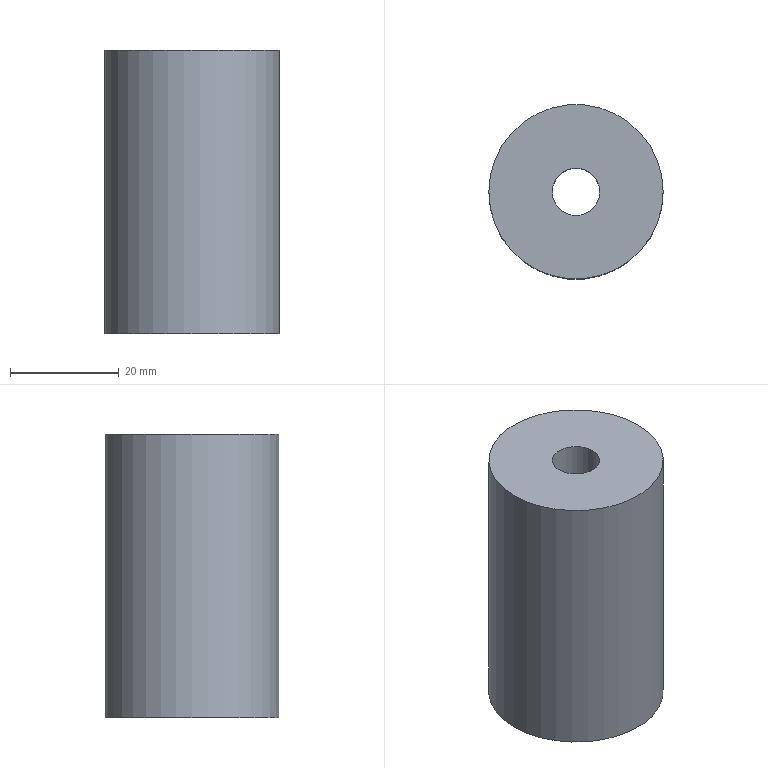Part | STEP file | 1_id1474_x_t | 1 solid | 6 faces | box 32 x 32 x 52.035 mm | volume 37231 mm3 | cylinder 3 | plane 3 | commonest cylinder face diameters 8.7 x1 15 x1 32 x1
STEP:
#1=CARTESIAN_POINT('',(0.,0.,0.));
#2=DIRECTION('',(0.,0.,1.));
#3=DIRECTION('',(1.,0.,0.));
#4=AXIS2_PLACEMENT_3D('',#1,#2,#3);
#5=CARTESIAN_POINT('',(238.925,-3.5,100.11));
#6=VERTEX_POINT('',#5);
#7=CARTESIAN_POINT('',(206.925,-3.5,100.11));
#8=VERTEX_POINT('',#7);
#9=CARTESIAN_POINT('',(222.925,-3.5,100.11));
#10=DIRECTION('',(0.,0.,1.));
#11=DIRECTION('',(-1.,0.,0.));
#12=AXIS2_PLACEMENT_3D('',#9,#10,#11);
#13=CIRCLE('',#12,16.);
#14=CARTESIAN_POINT('',(222.925,-3.5,98.075));
#15=DIRECTION('',(0.,0.,1.));
#16=DIRECTION('',(1.,0.,0.));
#17=AXIS2_PLACEMENT_3D('',#14,#15,#16);
#18=CYLINDRICAL_SURFACE('',#17,16.);
#19=CARTESIAN_POINT('',(-3.142,2.035));
#20=DIRECTION('',(1.,0.));
#21=VECTOR('',#20,1.);
#22=LINE('',#19,#21);
#23=(GEOMETRIC_REPRESENTATION_CONTEXT(2)PARAMETRIC_REPRESENTATION_CONTEXT()REPRESENTATION_CONTEXT('',''));
#24=DEFINITIONAL_REPRESENTATION('',(#22),#23);
#25=PCURVE('',#18,#24);
#26=CARTESIAN_POINT('',(239.613,177.297,100.11));
#27=DIRECTION('',(0.,0.,1.));
#28=DIRECTION('',(1.,0.,0.));
#29=AXIS2_PLACEMENT_3D('',#26,#27,#28);
#30=PLANE('',#29);
#31=CARTESIAN_POINT('',(-16.688,-180.797));
#32=DIRECTION('',(-1.,0.));
#33=AXIS2_PLACEMENT_2D('',#31,#32);
#34=CIRCLE('',#33,16.);
#35=(GEOMETRIC_REPRESENTATION_CONTEXT(2)PARAMETRIC_REPRESENTATION_CONTEXT()REPRESENTATION_CONTEXT('',''));
#36=DEFINITIONAL_REPRESENTATION('',(#34),#35);
#37=PCURVE('',#30,#36);
#38=SURFACE_CURVE('',#13,(#25,#37),.PCURVE_S1.);
#39=EDGE_CURVE('',#6,#8,#38,.T.);
#40=ORIENTED_EDGE('',*,*,#39,.F.);
#41=CARTESIAN_POINT('',(238.925,-3.5,48.075));
#42=VERTEX_POINT('',#41);
#43=CARTESIAN_POINT('',(238.925,-3.5,48.075));
#44=CARTESIAN_POINT('',(238.925,-3.5,100.11));
#45=B_SPLINE_CURVE_WITH_KNOTS('',1,(#43,#44),.UNSPECIFIED.,.F.,.F.,(2,2),(-50.,2.035),.PIECEWISE_BEZIER_KNOTS.);
#46=CARTESIAN_POINT('',(0.,0.));
#47=DIRECTION('',(0.,1.));
#48=VECTOR('',#47,1.);
#49=LINE('',#46,#48);
#50=(GEOMETRIC_REPRESENTATION_CONTEXT(2)PARAMETRIC_REPRESENTATION_CONTEXT()REPRESENTATION_CONTEXT('',''));
#51=DEFINITIONAL_REPRESENTATION('',(#49),#50);
#52=PCURVE('',#18,#51);
#53=CARTESIAN_POINT('',(6.283,0.));
#54=DIRECTION('',(0.,1.));
#55=VECTOR('',#54,1.);
#56=LINE('',#53,#55);
#57=(GEOMETRIC_REPRESENTATION_CONTEXT(2)PARAMETRIC_REPRESENTATION_CONTEXT()REPRESENTATION_CONTEXT('',''));
#58=DEFINITIONAL_REPRESENTATION('',(#56),#57);
#59=PCURVE('',#18,#58);
#60=SEAM_CURVE('',#45,(#52,#59),.PCURVE_S1.);
#61=EDGE_CURVE('',#42,#6,#60,.T.);
#62=ORIENTED_EDGE('',*,*,#61,.F.);
#63=CARTESIAN_POINT('',(222.925,-3.5,48.075));
#64=DIRECTION('',(0.,0.,-1.));
#65=DIRECTION('',(1.,0.,0.));
#66=AXIS2_PLACEMENT_3D('',#63,#64,#65);
#67=CIRCLE('',#66,16.);
#68=CARTESIAN_POINT('',(6.283,-50.));
#69=DIRECTION('',(-1.,0.));
#70=VECTOR('',#69,1.);
#71=LINE('',#68,#70);
#72=(GEOMETRIC_REPRESENTATION_CONTEXT(2)PARAMETRIC_REPRESENTATION_CONTEXT()REPRESENTATION_CONTEXT('',''));
#73=DEFINITIONAL_REPRESENTATION('',(#71),#72);
#74=PCURVE('',#18,#73);
#75=CARTESIAN_POINT('',(222.925,-3.5,48.075));
#76=DIRECTION('',(0.,0.,1.));
#77=DIRECTION('',(-1.,0.,0.));
#78=AXIS2_PLACEMENT_3D('',#75,#76,#77);
#79=PLANE('',#78);
#80=CARTESIAN_POINT('',(-16.,0.));
#81=CARTESIAN_POINT('',(-16.,27.713));
#82=CARTESIAN_POINT('',(8.,13.856));
#83=CARTESIAN_POINT('',(32.,0.));
#84=CARTESIAN_POINT('',(8.,-13.856));
#85=CARTESIAN_POINT('',(-16.,-27.713));
#86=CARTESIAN_POINT('',(-16.,0.));
#87=(BOUNDED_CURVE()B_SPLINE_CURVE(2,(#80,#81,#82,#83,#84,#85,#86),.UNSPECIFIED.,.T.,.F.)B_SPLINE_CURVE_WITH_KNOTS((1,2,2,2,2,1),(-2.094,0.,2.094,4.189,6.283,8.378),.UNSPECIFIED.)CURVE()GEOMETRIC_REPRESENTATION_ITEM()RATIONAL_B_SPLINE_CURVE((1.,0.5,1.,0.5,1.,0.5,1.))REPRESENTATION_ITEM(''));
#88=(GEOMETRIC_REPRESENTATION_CONTEXT(2)PARAMETRIC_REPRESENTATION_CONTEXT()REPRESENTATION_CONTEXT('',''));
#89=DEFINITIONAL_REPRESENTATION('',(#87),#88);
#90=PCURVE('',#79,#89);
#91=SURFACE_CURVE('',#67,(#74,#90),.PCURVE_S1.);
#92=EDGE_CURVE('',#42,#42,#91,.T.);
#93=ORIENTED_EDGE('',*,*,#92,.F.);
#94=ORIENTED_EDGE('',*,*,#61,.T.);
#95=CARTESIAN_POINT('',(222.925,-3.5,100.11));
#96=DIRECTION('',(0.,0.,1.));
#97=DIRECTION('',(-1.,0.,0.));
#98=AXIS2_PLACEMENT_3D('',#95,#96,#97);
#99=CIRCLE('',#98,16.);
#100=CARTESIAN_POINT('',(3.142,2.035));
#101=DIRECTION('',(1.,0.));
#102=VECTOR('',#101,1.);
#103=LINE('',#100,#102);
#104=(GEOMETRIC_REPRESENTATION_CONTEXT(2)PARAMETRIC_REPRESENTATION_CONTEXT()REPRESENTATION_CONTEXT('',''));
#105=DEFINITIONAL_REPRESENTATION('',(#103),#104);
#106=PCURVE('',#18,#105);
#107=CARTESIAN_POINT('',(-16.688,-180.797));
#108=DIRECTION('',(-1.,0.));
#109=AXIS2_PLACEMENT_2D('',#107,#108);
#110=CIRCLE('',#109,16.);
#111=(GEOMETRIC_REPRESENTATION_CONTEXT(2)PARAMETRIC_REPRESENTATION_CONTEXT()REPRESENTATION_CONTEXT('',''));
#112=DEFINITIONAL_REPRESENTATION('',(#110),#111);
#113=PCURVE('',#30,#112);
#114=SURFACE_CURVE('',#99,(#106,#113),.PCURVE_S1.);
#115=EDGE_CURVE('',#8,#6,#114,.T.);
#116=ORIENTED_EDGE('',*,*,#115,.F.);
#117=EDGE_LOOP('',(#40,#62,#93,#94,#116));
#118=FACE_BOUND('',#117,.T.);
#119=ADVANCED_FACE('',(#118),#18,.T.);
#120=ORIENTED_EDGE('',*,*,#92,.T.);
#121=EDGE_LOOP('',(#120));
#122=FACE_BOUND('',#121,.T.);
#123=CARTESIAN_POINT('',(215.425,-3.5,48.075));
#124=VERTEX_POINT('',#123);
#125=CARTESIAN_POINT('',(222.925,-3.5,48.075));
#126=DIRECTION('',(0.,0.,1.));
#127=DIRECTION('',(-1.,0.,0.));
#128=AXIS2_PLACEMENT_3D('',#125,#126,#127);
#129=CIRCLE('',#128,7.5);
#130=CARTESIAN_POINT('',(0.,0.));
#131=DIRECTION('',(1.,0.));
#132=AXIS2_PLACEMENT_2D('',#130,#131);
#133=CIRCLE('',#132,7.5);
#134=(GEOMETRIC_REPRESENTATION_CONTEXT(2)PARAMETRIC_REPRESENTATION_CONTEXT()REPRESENTATION_CONTEXT('',''));
#135=DEFINITIONAL_REPRESENTATION('',(#133),#134);
#136=PCURVE('',#79,#135);
#137=CARTESIAN_POINT('',(222.925,-3.5,61.075));
#138=DIRECTION('',(0.,0.,1.));
#139=DIRECTION('',(1.,0.,0.));
#140=AXIS2_PLACEMENT_3D('',#137,#138,#139);
#141=CYLINDRICAL_SURFACE('',#140,7.5);
#142=CARTESIAN_POINT('',(3.142,-13.));
#143=DIRECTION('',(1.,0.));
#144=VECTOR('',#143,1.);
#145=LINE('',#142,#144);
#146=(GEOMETRIC_REPRESENTATION_CONTEXT(2)PARAMETRIC_REPRESENTATION_CONTEXT()REPRESENTATION_CONTEXT('',''));
#147=DEFINITIONAL_REPRESENTATION('',(#145),#146);
#148=PCURVE('',#141,#147);
#149=SURFACE_CURVE('',#129,(#136,#148),.PCURVE_S1.);
#150=EDGE_CURVE('',#124,#124,#149,.T.);
#151=ORIENTED_EDGE('',*,*,#150,.T.);
#152=EDGE_LOOP('',(#151));
#153=FACE_BOUND('',#152,.T.);
#154=ADVANCED_FACE('',(#122,#153),#79,.F.);
#155=ORIENTED_EDGE('',*,*,#115,.T.);
#156=ORIENTED_EDGE('',*,*,#39,.T.);
#157=EDGE_LOOP('',(#155,#156));
#158=FACE_BOUND('',#157,.T.);
#159=CARTESIAN_POINT('',(218.575,-3.5,100.11));
#160=VERTEX_POINT('',#159);
#161=CARTESIAN_POINT('',(227.275,-3.5,100.11));
#162=VERTEX_POINT('',#161);
#163=CARTESIAN_POINT('',(222.925,-3.5,100.11));
#164=DIRECTION('',(0.,0.,-1.));
#165=DIRECTION('',(-1.,0.,0.));
#166=AXIS2_PLACEMENT_3D('',#163,#164,#165);
#167=CIRCLE('',#166,4.35);
#168=CARTESIAN_POINT('',(-21.038,-180.797));
#169=CARTESIAN_POINT('',(-21.038,-173.262));
#170=CARTESIAN_POINT('',(-14.513,-177.029));
#171=CARTESIAN_POINT('',(-7.988,-180.797));
#172=CARTESIAN_POINT('',(-14.513,-184.564));
#173=CARTESIAN_POINT('',(-21.038,-188.331));
#174=CARTESIAN_POINT('',(-21.038,-180.797));
#175=(BOUNDED_CURVE()B_SPLINE_CURVE(2,(#168,#169,#170,#171,#172,#173,#174),.UNSPECIFIED.,.T.,.F.)B_SPLINE_CURVE_WITH_KNOTS((1,2,2,2,2,1),(-2.094,0.,2.094,4.189,6.283,8.378),.UNSPECIFIED.)CURVE()GEOMETRIC_REPRESENTATION_ITEM()RATIONAL_B_SPLINE_CURVE((1.,0.5,1.,0.5,1.,0.5,1.))REPRESENTATION_ITEM(''));
#176=(GEOMETRIC_REPRESENTATION_CONTEXT(2)PARAMETRIC_REPRESENTATION_CONTEXT()REPRESENTATION_CONTEXT('',''));
#177=DEFINITIONAL_REPRESENTATION('',(#175),#176);
#178=PCURVE('',#30,#177);
#179=CARTESIAN_POINT('',(222.925,-3.5,98.575));
#180=DIRECTION('',(0.,0.,1.));
#181=DIRECTION('',(1.,0.,0.));
#182=AXIS2_PLACEMENT_3D('',#179,#180,#181);
#183=CYLINDRICAL_SURFACE('',#182,4.35);
#184=CARTESIAN_POINT('',(3.142,1.535));
#185=DIRECTION('',(-1.,0.));
#186=VECTOR('',#185,1.);
#187=LINE('',#184,#186);
#188=(GEOMETRIC_REPRESENTATION_CONTEXT(2)PARAMETRIC_REPRESENTATION_CONTEXT()REPRESENTATION_CONTEXT('',''));
#189=DEFINITIONAL_REPRESENTATION('',(#187),#188);
#190=PCURVE('',#183,#189);
#191=SURFACE_CURVE('',#167,(#178,#190),.PCURVE_S1.);
#192=EDGE_CURVE('',#160,#162,#191,.T.);
#193=ORIENTED_EDGE('',*,*,#192,.T.);
#194=CARTESIAN_POINT('',(222.925,-3.5,100.11));
#195=DIRECTION('',(0.,0.,-1.));
#196=DIRECTION('',(-1.,0.,0.));
#197=AXIS2_PLACEMENT_3D('',#194,#195,#196);
#198=CIRCLE('',#197,4.35);
#199=CARTESIAN_POINT('',(-21.038,-180.797));
#200=CARTESIAN_POINT('',(-21.038,-173.262));
#201=CARTESIAN_POINT('',(-14.513,-177.029));
#202=CARTESIAN_POINT('',(-7.988,-180.797));
#203=CARTESIAN_POINT('',(-14.513,-184.564));
#204=CARTESIAN_POINT('',(-21.038,-188.331));
#205=CARTESIAN_POINT('',(-21.038,-180.797));
#206=(BOUNDED_CURVE()B_SPLINE_CURVE(2,(#199,#200,#201,#202,#203,#204,#205),.UNSPECIFIED.,.T.,.F.)B_SPLINE_CURVE_WITH_KNOTS((1,2,2,2,2,1),(-2.094,0.,2.094,4.189,6.283,8.378),.UNSPECIFIED.)CURVE()GEOMETRIC_REPRESENTATION_ITEM()RATIONAL_B_SPLINE_CURVE((1.,0.5,1.,0.5,1.,0.5,1.))REPRESENTATION_ITEM(''));
#207=(GEOMETRIC_REPRESENTATION_CONTEXT(2)PARAMETRIC_REPRESENTATION_CONTEXT()REPRESENTATION_CONTEXT('',''));
#208=DEFINITIONAL_REPRESENTATION('',(#206),#207);
#209=PCURVE('',#30,#208);
#210=CARTESIAN_POINT('',(9.425,1.535));
#211=DIRECTION('',(-1.,0.));
#212=VECTOR('',#211,1.);
#213=LINE('',#210,#212);
#214=(GEOMETRIC_REPRESENTATION_CONTEXT(2)PARAMETRIC_REPRESENTATION_CONTEXT()REPRESENTATION_CONTEXT('',''));
#215=DEFINITIONAL_REPRESENTATION('',(#213),#214);
#216=PCURVE('',#183,#215);
#217=SURFACE_CURVE('',#198,(#209,#216),.PCURVE_S1.);
#218=EDGE_CURVE('',#162,#160,#217,.T.);
#219=ORIENTED_EDGE('',*,*,#218,.T.);
#220=EDGE_LOOP('',(#193,#219));
#221=FACE_BOUND('',#220,.T.);
#222=ADVANCED_FACE('',(#158,#221),#30,.T.);
#223=ORIENTED_EDGE('',*,*,#192,.T.);
#224=CARTESIAN_POINT('',(227.275,-3.5,61.075));
#225=VERTEX_POINT('',#224);
#226=CARTESIAN_POINT('',(227.275,-3.5,61.075));
#227=CARTESIAN_POINT('',(227.275,-3.5,100.11));
#228=B_SPLINE_CURVE_WITH_KNOTS('',1,(#226,#227),.UNSPECIFIED.,.F.,.F.,(2,2),(-37.5,1.535),.PIECEWISE_BEZIER_KNOTS.);
#229=CARTESIAN_POINT('',(0.,0.));
#230=DIRECTION('',(0.,1.));
#231=VECTOR('',#230,1.);
#232=LINE('',#229,#231);
#233=(GEOMETRIC_REPRESENTATION_CONTEXT(2)PARAMETRIC_REPRESENTATION_CONTEXT()REPRESENTATION_CONTEXT('',''));
#234=DEFINITIONAL_REPRESENTATION('',(#232),#233);
#235=PCURVE('',#183,#234);
#236=CARTESIAN_POINT('',(6.283,0.));
#237=DIRECTION('',(0.,1.));
#238=VECTOR('',#237,1.);
#239=LINE('',#236,#238);
#240=(GEOMETRIC_REPRESENTATION_CONTEXT(2)PARAMETRIC_REPRESENTATION_CONTEXT()REPRESENTATION_CONTEXT('',''));
#241=DEFINITIONAL_REPRESENTATION('',(#239),#240);
#242=PCURVE('',#183,#241);
#243=SEAM_CURVE('',#228,(#235,#242),.PCURVE_S1.);
#244=EDGE_CURVE('',#225,#162,#243,.T.);
#245=ORIENTED_EDGE('',*,*,#244,.F.);
#246=CARTESIAN_POINT('',(222.925,-3.5,61.075));
#247=DIRECTION('',(0.,0.,1.));
#248=DIRECTION('',(1.,0.,0.));
#249=AXIS2_PLACEMENT_3D('',#246,#247,#248);
#250=CIRCLE('',#249,4.35);
#251=CARTESIAN_POINT('',(0.,-37.5));
#252=DIRECTION('',(1.,0.));
#253=VECTOR('',#252,1.);
#254=LINE('',#251,#253);
#255=(GEOMETRIC_REPRESENTATION_CONTEXT(2)PARAMETRIC_REPRESENTATION_CONTEXT()REPRESENTATION_CONTEXT('',''));
#256=DEFINITIONAL_REPRESENTATION('',(#254),#255);
#257=PCURVE('',#183,#256);
#258=CARTESIAN_POINT('',(222.925,-3.5,61.075));
#259=DIRECTION('',(0.,0.,1.));
#260=DIRECTION('',(-1.,0.,0.));
#261=AXIS2_PLACEMENT_3D('',#258,#259,#260);
#262=PLANE('',#261);
#263=CARTESIAN_POINT('',(0.,0.));
#264=DIRECTION('',(-1.,0.));
#265=AXIS2_PLACEMENT_2D('',#263,#264);
#266=CIRCLE('',#265,4.35);
#267=(GEOMETRIC_REPRESENTATION_CONTEXT(2)PARAMETRIC_REPRESENTATION_CONTEXT()REPRESENTATION_CONTEXT('',''));
#268=DEFINITIONAL_REPRESENTATION('',(#266),#267);
#269=PCURVE('',#262,#268);
#270=SURFACE_CURVE('',#250,(#257,#269),.PCURVE_S1.);
#271=EDGE_CURVE('',#225,#225,#270,.T.);
#272=ORIENTED_EDGE('',*,*,#271,.T.);
#273=ORIENTED_EDGE('',*,*,#244,.T.);
#274=ORIENTED_EDGE('',*,*,#218,.T.);
#275=EDGE_LOOP('',(#223,#245,#272,#273,#274));
#276=FACE_BOUND('',#275,.F.);
#277=ADVANCED_FACE('',(#276),#183,.F.);
#278=CARTESIAN_POINT('',(215.425,-3.5,61.075));
#279=VERTEX_POINT('',#278);
#280=CARTESIAN_POINT('',(222.925,-3.5,61.075));
#281=DIRECTION('',(0.,0.,-1.));
#282=DIRECTION('',(-1.,0.,0.));
#283=AXIS2_PLACEMENT_3D('',#280,#281,#282);
#284=CIRCLE('',#283,7.5);
#285=CARTESIAN_POINT('',(7.5,0.));
#286=CARTESIAN_POINT('',(7.5,-12.99));
#287=CARTESIAN_POINT('',(-3.75,-6.495));
#288=CARTESIAN_POINT('',(-15.,0.));
#289=CARTESIAN_POINT('',(-3.75,6.495));
#290=CARTESIAN_POINT('',(7.5,12.99));
#291=CARTESIAN_POINT('',(7.5,0.));
#292=(BOUNDED_CURVE()B_SPLINE_CURVE(2,(#285,#286,#287,#288,#289,#290,#291),.UNSPECIFIED.,.T.,.F.)B_SPLINE_CURVE_WITH_KNOTS((1,2,2,2,2,1),(-2.094,0.,2.094,4.189,6.283,8.378),.UNSPECIFIED.)CURVE()GEOMETRIC_REPRESENTATION_ITEM()RATIONAL_B_SPLINE_CURVE((1.,0.5,1.,0.5,1.,0.5,1.))REPRESENTATION_ITEM(''));
#293=(GEOMETRIC_REPRESENTATION_CONTEXT(2)PARAMETRIC_REPRESENTATION_CONTEXT()REPRESENTATION_CONTEXT('',''));
#294=DEFINITIONAL_REPRESENTATION('',(#292),#293);
#295=PCURVE('',#262,#294);
#296=CARTESIAN_POINT('',(9.425,0.));
#297=DIRECTION('',(-1.,0.));
#298=VECTOR('',#297,1.);
#299=LINE('',#296,#298);
#300=(GEOMETRIC_REPRESENTATION_CONTEXT(2)PARAMETRIC_REPRESENTATION_CONTEXT()REPRESENTATION_CONTEXT('',''));
#301=DEFINITIONAL_REPRESENTATION('',(#299),#300);
#302=PCURVE('',#141,#301);
#303=SURFACE_CURVE('',#284,(#295,#302),.PCURVE_S1.);
#304=EDGE_CURVE('',#279,#279,#303,.T.);
#305=ORIENTED_EDGE('',*,*,#304,.T.);
#306=EDGE_LOOP('',(#305));
#307=FACE_BOUND('',#306,.T.);
#308=ORIENTED_EDGE('',*,*,#271,.T.);
#309=EDGE_LOOP('',(#308));
#310=FACE_BOUND('',#309,.T.);
#311=ADVANCED_FACE('',(#307,#310),#262,.F.);
#312=ORIENTED_EDGE('',*,*,#304,.T.);
#313=CARTESIAN_POINT('',(215.425,-3.5,48.075));
#314=CARTESIAN_POINT('',(215.425,-3.5,61.075));
#315=B_SPLINE_CURVE_WITH_KNOTS('',1,(#313,#314),.UNSPECIFIED.,.F.,.F.,(2,2),(-13.,0.),.PIECEWISE_BEZIER_KNOTS.);
#316=CARTESIAN_POINT('',(3.142,0.));
#317=DIRECTION('',(0.,1.));
#318=VECTOR('',#317,1.);
#319=LINE('',#316,#318);
#320=(GEOMETRIC_REPRESENTATION_CONTEXT(2)PARAMETRIC_REPRESENTATION_CONTEXT()REPRESENTATION_CONTEXT('',''));
#321=DEFINITIONAL_REPRESENTATION('',(#319),#320);
#322=PCURVE('',#141,#321);
#323=CARTESIAN_POINT('',(9.425,0.));
#324=DIRECTION('',(0.,1.));
#325=VECTOR('',#324,1.);
#326=LINE('',#323,#325);
#327=(GEOMETRIC_REPRESENTATION_CONTEXT(2)PARAMETRIC_REPRESENTATION_CONTEXT()REPRESENTATION_CONTEXT('',''));
#328=DEFINITIONAL_REPRESENTATION('',(#326),#327);
#329=PCURVE('',#141,#328);
#330=SEAM_CURVE('',#315,(#322,#329),.PCURVE_S1.);
#331=EDGE_CURVE('',#124,#279,#330,.T.);
#332=ORIENTED_EDGE('',*,*,#331,.F.);
#333=ORIENTED_EDGE('',*,*,#150,.T.);
#334=ORIENTED_EDGE('',*,*,#331,.T.);
#335=EDGE_LOOP('',(#312,#332,#333,#334));
#336=FACE_BOUND('',#335,.F.);
#337=ADVANCED_FACE('',(#336),#141,.F.);
#338=CLOSED_SHELL('',(#119,#154,#222,#277,#311,#337));
#339=MANIFOLD_SOLID_BREP('',#338);
#340=(LENGTH_UNIT()NAMED_UNIT(*)SI_UNIT(.MILLI.,.METRE.));
#341=UNCERTAINTY_MEASURE_WITH_UNIT(LENGTH_MEASURE(0.000005),#340,'','');
#342=(NAMED_UNIT(*)PLANE_ANGLE_UNIT()SI_UNIT($,.RADIAN.));
#343=(NAMED_UNIT(*)SI_UNIT($,.STERADIAN.)SOLID_ANGLE_UNIT());
#344=(GEOMETRIC_REPRESENTATION_CONTEXT(3)GLOBAL_UNCERTAINTY_ASSIGNED_CONTEXT((#341))GLOBAL_UNIT_ASSIGNED_CONTEXT((#340,#342,#343))REPRESENTATION_CONTEXT('',''));
#345=ADVANCED_BREP_SHAPE_REPRESENTATION('',(#4,#339),#344);